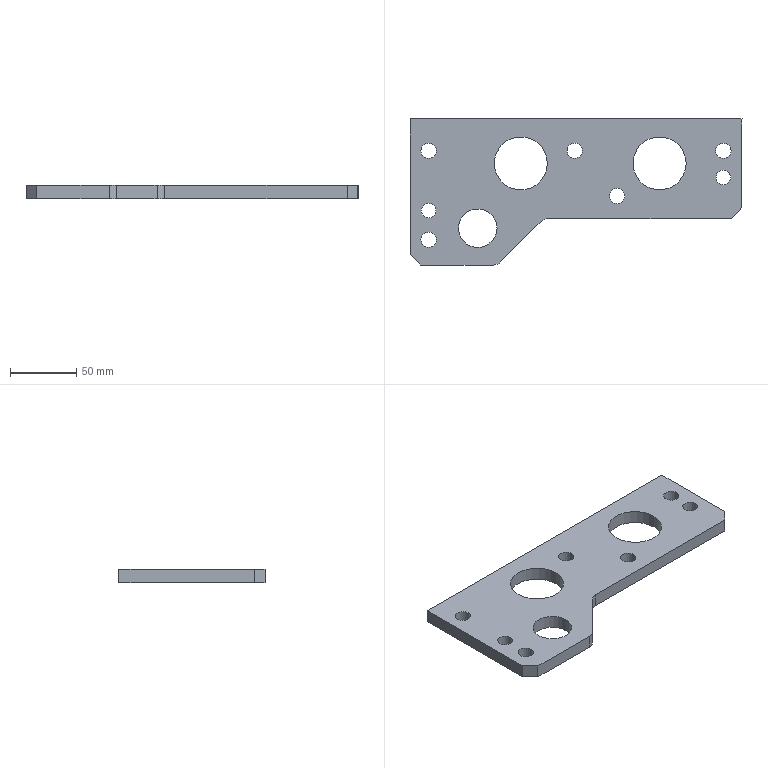Part | STEP file | lll_id4266_x_t | 1 solid | 22 faces | box 250 x 110 x 10 mm | volume 177245 mm3 | cylinder 12 | plane 10 | commonest cylinder face diameters 11.509 x5 11 x2 16 x2 40 x2 29 x1
STEP:
#1=CARTESIAN_POINT('',(3214.622,127.75,-35.));
#2=VERTEX_POINT('',#1);
#3=CARTESIAN_POINT('',(3214.622,127.75,-45.));
#4=VERTEX_POINT('',#3);
#5=CARTESIAN_POINT('',(3214.622,127.75,-35.));
#6=DIRECTION('',(0.,0.,-1.));
#7=VECTOR('',#6,1.);
#8=LINE('',#5,#7);
#9=EDGE_CURVE('',#2,#4,#8,.T.);
#10=ORIENTED_EDGE('',*,*,#9,.F.);
#11=CARTESIAN_POINT('',(3159.935,127.75,-35.));
#12=VERTEX_POINT('',#11);
#13=CARTESIAN_POINT('',(3266.435,127.75,-35.));
#14=DIRECTION('',(1.,0.,0.));
#15=VECTOR('',#14,1.);
#16=LINE('',#13,#15);
#17=EDGE_CURVE('',#12,#2,#16,.T.);
#18=ORIENTED_EDGE('',*,*,#17,.F.);
#19=CARTESIAN_POINT('',(3159.935,127.75,-45.));
#20=VERTEX_POINT('',#19);
#21=CARTESIAN_POINT('',(3159.935,127.75,-35.));
#22=DIRECTION('',(0.,0.,-1.));
#23=VECTOR('',#22,1.);
#24=LINE('',#21,#23);
#25=EDGE_CURVE('',#12,#20,#24,.T.);
#26=ORIENTED_EDGE('',*,*,#25,.T.);
#27=CARTESIAN_POINT('',(3266.435,127.75,-45.));
#28=DIRECTION('',(1.,0.,0.));
#29=VECTOR('',#28,1.);
#30=LINE('',#27,#29);
#31=EDGE_CURVE('',#20,#4,#30,.T.);
#32=ORIENTED_EDGE('',*,*,#31,.T.);
#33=EDGE_LOOP('',(#10,#18,#26,#32));
#34=FACE_OUTER_BOUND('',#33,.T.);
#35=CARTESIAN_POINT('',(3266.435,127.75,-35.));
#36=DIRECTION('',(0.,-1.,0.));
#37=DIRECTION('',(-1.,0.,0.));
#38=AXIS2_PLACEMENT_3D('',#35,#36,#37);
#39=PLANE('',#38);
#40=ADVANCED_FACE('',(#34),#39,.T.);
#41=ORIENTED_EDGE('',*,*,#25,.F.);
#42=CARTESIAN_POINT('',(3151.935,135.75,-35.));
#43=VERTEX_POINT('',#42);
#44=CARTESIAN_POINT('',(3169.435,118.25,-35.));
#45=DIRECTION('',(-0.7071,0.7071,0.));
#46=VECTOR('',#45,1.);
#47=LINE('',#44,#46);
#48=EDGE_CURVE('',#12,#43,#47,.T.);
#49=ORIENTED_EDGE('',*,*,#48,.T.);
#50=CARTESIAN_POINT('',(3151.935,135.75,-45.));
#51=VERTEX_POINT('',#50);
#52=CARTESIAN_POINT('',(3151.935,135.75,-35.));
#53=DIRECTION('',(0.,0.,-1.));
#54=VECTOR('',#53,1.);
#55=LINE('',#52,#54);
#56=EDGE_CURVE('',#43,#51,#55,.T.);
#57=ORIENTED_EDGE('',*,*,#56,.T.);
#58=CARTESIAN_POINT('',(3169.435,118.25,-45.));
#59=DIRECTION('',(-0.7071,0.7071,0.));
#60=VECTOR('',#59,1.);
#61=LINE('',#58,#60);
#62=EDGE_CURVE('',#20,#51,#61,.T.);
#63=ORIENTED_EDGE('',*,*,#62,.F.);
#64=EDGE_LOOP('',(#41,#49,#57,#63));
#65=FACE_OUTER_BOUND('',#64,.T.);
#66=CARTESIAN_POINT('',(3169.435,118.25,-35.));
#67=DIRECTION('',(-0.7071,-0.7071,0.));
#68=DIRECTION('',(-0.7071,0.7071,0.));
#69=AXIS2_PLACEMENT_3D('',#66,#67,#68);
#70=PLANE('',#69);
#71=ADVANCED_FACE('',(#65),#70,.T.);
#72=ORIENTED_EDGE('',*,*,#56,.F.);
#73=CARTESIAN_POINT('',(3151.935,237.75,-35.));
#74=VERTEX_POINT('',#73);
#75=CARTESIAN_POINT('',(3151.935,215.25,-35.));
#76=DIRECTION('',(0.,-1.,0.));
#77=VECTOR('',#76,1.);
#78=LINE('',#75,#77);
#79=EDGE_CURVE('',#74,#43,#78,.T.);
#80=ORIENTED_EDGE('',*,*,#79,.F.);
#81=CARTESIAN_POINT('',(3151.935,237.75,-45.));
#82=VERTEX_POINT('',#81);
#83=CARTESIAN_POINT('',(3151.935,237.75,-35.));
#84=DIRECTION('',(0.,0.,-1.));
#85=VECTOR('',#84,1.);
#86=LINE('',#83,#85);
#87=EDGE_CURVE('',#74,#82,#86,.T.);
#88=ORIENTED_EDGE('',*,*,#87,.T.);
#89=CARTESIAN_POINT('',(3151.935,215.25,-45.));
#90=DIRECTION('',(0.,-1.,0.));
#91=VECTOR('',#90,1.);
#92=LINE('',#89,#91);
#93=EDGE_CURVE('',#82,#51,#92,.T.);
#94=ORIENTED_EDGE('',*,*,#93,.T.);
#95=EDGE_LOOP('',(#72,#80,#88,#94));
#96=FACE_OUTER_BOUND('',#95,.T.);
#97=CARTESIAN_POINT('',(3151.935,215.25,-35.));
#98=DIRECTION('',(1.,0.,0.));
#99=DIRECTION('',(0.,-1.,0.));
#100=AXIS2_PLACEMENT_3D('',#97,#98,#99);
#101=PLANE('',#100);
#102=ADVANCED_FACE('',(#96),#101,.F.);
#103=ORIENTED_EDGE('',*,*,#87,.F.);
#104=CARTESIAN_POINT('',(3401.935,237.75,-35.));
#105=VERTEX_POINT('',#104);
#106=CARTESIAN_POINT('',(3266.435,237.75,-35.));
#107=DIRECTION('',(-1.,0.,0.));
#108=VECTOR('',#107,1.);
#109=LINE('',#106,#108);
#110=EDGE_CURVE('',#105,#74,#109,.T.);
#111=ORIENTED_EDGE('',*,*,#110,.F.);
#112=CARTESIAN_POINT('',(3401.935,237.75,-45.));
#113=VERTEX_POINT('',#112);
#114=CARTESIAN_POINT('',(3401.935,237.75,-35.));
#115=DIRECTION('',(0.,0.,-1.));
#116=VECTOR('',#115,1.);
#117=LINE('',#114,#116);
#118=EDGE_CURVE('',#105,#113,#117,.T.);
#119=ORIENTED_EDGE('',*,*,#118,.T.);
#120=CARTESIAN_POINT('',(3266.435,237.75,-45.));
#121=DIRECTION('',(-1.,0.,0.));
#122=VECTOR('',#121,1.);
#123=LINE('',#120,#122);
#124=EDGE_CURVE('',#113,#82,#123,.T.);
#125=ORIENTED_EDGE('',*,*,#124,.T.);
#126=EDGE_LOOP('',(#103,#111,#119,#125));
#127=FACE_OUTER_BOUND('',#126,.T.);
#128=CARTESIAN_POINT('',(3266.435,237.75,-35.));
#129=DIRECTION('',(0.,-1.,0.));
#130=DIRECTION('',(-1.,0.,0.));
#131=AXIS2_PLACEMENT_3D('',#128,#129,#130);
#132=PLANE('',#131);
#133=ADVANCED_FACE('',(#127),#132,.F.);
#134=ORIENTED_EDGE('',*,*,#118,.F.);
#135=CARTESIAN_POINT('',(3401.935,170.75,-35.));
#136=VERTEX_POINT('',#135);
#137=CARTESIAN_POINT('',(3401.935,215.25,-35.));
#138=DIRECTION('',(0.,1.,0.));
#139=VECTOR('',#138,1.);
#140=LINE('',#137,#139);
#141=EDGE_CURVE('',#136,#105,#140,.T.);
#142=ORIENTED_EDGE('',*,*,#141,.F.);
#143=CARTESIAN_POINT('',(3401.935,170.75,-45.));
#144=VERTEX_POINT('',#143);
#145=CARTESIAN_POINT('',(3401.935,170.75,-35.));
#146=DIRECTION('',(0.,0.,-1.));
#147=VECTOR('',#146,1.);
#148=LINE('',#145,#147);
#149=EDGE_CURVE('',#136,#144,#148,.T.);
#150=ORIENTED_EDGE('',*,*,#149,.T.);
#151=CARTESIAN_POINT('',(3401.935,215.25,-45.));
#152=DIRECTION('',(0.,1.,0.));
#153=VECTOR('',#152,1.);
#154=LINE('',#151,#153);
#155=EDGE_CURVE('',#144,#113,#154,.T.);
#156=ORIENTED_EDGE('',*,*,#155,.T.);
#157=EDGE_LOOP('',(#134,#142,#150,#156));
#158=FACE_OUTER_BOUND('',#157,.T.);
#159=CARTESIAN_POINT('',(3401.935,215.25,-35.));
#160=DIRECTION('',(-1.,0.,0.));
#161=DIRECTION('',(0.,1.,0.));
#162=AXIS2_PLACEMENT_3D('',#159,#160,#161);
#163=PLANE('',#162);
#164=ADVANCED_FACE('',(#158),#163,.F.);
#165=ORIENTED_EDGE('',*,*,#149,.F.);
#166=CARTESIAN_POINT('',(3393.935,162.75,-35.));
#167=VERTEX_POINT('',#166);
#168=CARTESIAN_POINT('',(3356.435,125.25,-35.));
#169=DIRECTION('',(-0.7071,-0.7071,0.));
#170=VECTOR('',#169,1.);
#171=LINE('',#168,#170);
#172=EDGE_CURVE('',#136,#167,#171,.T.);
#173=ORIENTED_EDGE('',*,*,#172,.T.);
#174=CARTESIAN_POINT('',(3393.935,162.75,-45.));
#175=VERTEX_POINT('',#174);
#176=CARTESIAN_POINT('',(3393.935,162.75,-35.));
#177=DIRECTION('',(0.,0.,-1.));
#178=VECTOR('',#177,1.);
#179=LINE('',#176,#178);
#180=EDGE_CURVE('',#167,#175,#179,.T.);
#181=ORIENTED_EDGE('',*,*,#180,.T.);
#182=CARTESIAN_POINT('',(3356.435,125.25,-45.));
#183=DIRECTION('',(-0.7071,-0.7071,0.));
#184=VECTOR('',#183,1.);
#185=LINE('',#182,#184);
#186=EDGE_CURVE('',#144,#175,#185,.T.);
#187=ORIENTED_EDGE('',*,*,#186,.F.);
#188=EDGE_LOOP('',(#165,#173,#181,#187));
#189=FACE_OUTER_BOUND('',#188,.T.);
#190=CARTESIAN_POINT('',(3356.435,125.25,-35.));
#191=DIRECTION('',(0.7071,-0.7071,0.));
#192=DIRECTION('',(-0.7071,-0.7071,0.));
#193=AXIS2_PLACEMENT_3D('',#190,#191,#192);
#194=PLANE('',#193);
#195=ADVANCED_FACE('',(#189),#194,.T.);
#196=ORIENTED_EDGE('',*,*,#180,.F.);
#197=CARTESIAN_POINT('',(3256.249,162.75,-35.));
#198=VERTEX_POINT('',#197);
#199=CARTESIAN_POINT('',(3266.435,162.75,-35.));
#200=DIRECTION('',(-1.,0.,0.));
#201=VECTOR('',#200,1.);
#202=LINE('',#199,#201);
#203=EDGE_CURVE('',#167,#198,#202,.T.);
#204=ORIENTED_EDGE('',*,*,#203,.T.);
#205=CARTESIAN_POINT('',(3256.249,162.75,-45.));
#206=VERTEX_POINT('',#205);
#207=CARTESIAN_POINT('',(3256.249,162.75,-35.));
#208=DIRECTION('',(0.,0.,-1.));
#209=VECTOR('',#208,1.);
#210=LINE('',#207,#209);
#211=EDGE_CURVE('',#198,#206,#210,.T.);
#212=ORIENTED_EDGE('',*,*,#211,.T.);
#213=CARTESIAN_POINT('',(3266.435,162.75,-45.));
#214=DIRECTION('',(-1.,0.,0.));
#215=VECTOR('',#214,1.);
#216=LINE('',#213,#215);
#217=EDGE_CURVE('',#175,#206,#216,.T.);
#218=ORIENTED_EDGE('',*,*,#217,.F.);
#219=EDGE_LOOP('',(#196,#204,#212,#218));
#220=FACE_OUTER_BOUND('',#219,.T.);
#221=CARTESIAN_POINT('',(3266.435,162.75,-35.));
#222=DIRECTION('',(0.,-1.,0.));
#223=DIRECTION('',(-1.,0.,0.));
#224=AXIS2_PLACEMENT_3D('',#221,#222,#223);
#225=PLANE('',#224);
#226=ADVANCED_FACE('',(#220),#225,.T.);
#227=ORIENTED_EDGE('',*,*,#211,.F.);
#228=CARTESIAN_POINT('',(3250.592,160.407,-35.));
#229=VERTEX_POINT('',#228);
#230=CARTESIAN_POINT('',(3256.249,154.75,-35.));
#231=DIRECTION('',(0.,0.,1.));
#232=DIRECTION('',(-1.,0.,0.));
#233=AXIS2_PLACEMENT_3D('',#230,#231,#232);
#234=CIRCLE('',#233,8.);
#235=EDGE_CURVE('',#198,#229,#234,.T.);
#236=ORIENTED_EDGE('',*,*,#235,.T.);
#237=CARTESIAN_POINT('',(3250.592,160.407,-45.));
#238=VERTEX_POINT('',#237);
#239=CARTESIAN_POINT('',(3250.592,160.407,-35.));
#240=DIRECTION('',(0.,0.,-1.));
#241=VECTOR('',#240,1.);
#242=LINE('',#239,#241);
#243=EDGE_CURVE('',#229,#238,#242,.T.);
#244=ORIENTED_EDGE('',*,*,#243,.T.);
#245=CARTESIAN_POINT('',(3256.249,154.75,-45.));
#246=DIRECTION('',(0.,0.,1.));
#247=DIRECTION('',(-1.,0.,0.));
#248=AXIS2_PLACEMENT_3D('',#245,#246,#247);
#249=CIRCLE('',#248,8.);
#250=EDGE_CURVE('',#206,#238,#249,.T.);
#251=ORIENTED_EDGE('',*,*,#250,.F.);
#252=EDGE_LOOP('',(#227,#236,#244,#251));
#253=FACE_OUTER_BOUND('',#252,.T.);
#254=CARTESIAN_POINT('',(3256.249,154.75,-35.));
#255=DIRECTION('',(0.,0.,-1.));
#256=DIRECTION('',(-1.,0.,0.));
#257=AXIS2_PLACEMENT_3D('',#254,#255,#256);
#258=CYLINDRICAL_SURFACE('',#257,8.);
#259=ADVANCED_FACE('',(#253),#258,.F.);
#260=ORIENTED_EDGE('',*,*,#243,.F.);
#261=CARTESIAN_POINT('',(3220.278,130.093,-35.));
#262=VERTEX_POINT('',#261);
#263=CARTESIAN_POINT('',(3285.935,195.75,-35.));
#264=DIRECTION('',(0.7071,0.7071,0.));
#265=VECTOR('',#264,1.);
#266=LINE('',#263,#265);
#267=EDGE_CURVE('',#262,#229,#266,.T.);
#268=ORIENTED_EDGE('',*,*,#267,.F.);
#269=CARTESIAN_POINT('',(3220.278,130.093,-45.));
#270=VERTEX_POINT('',#269);
#271=CARTESIAN_POINT('',(3220.278,130.093,-35.));
#272=DIRECTION('',(0.,0.,-1.));
#273=VECTOR('',#272,1.);
#274=LINE('',#271,#273);
#275=EDGE_CURVE('',#262,#270,#274,.T.);
#276=ORIENTED_EDGE('',*,*,#275,.T.);
#277=CARTESIAN_POINT('',(3285.935,195.75,-45.));
#278=DIRECTION('',(0.7071,0.7071,0.));
#279=VECTOR('',#278,1.);
#280=LINE('',#277,#279);
#281=EDGE_CURVE('',#270,#238,#280,.T.);
#282=ORIENTED_EDGE('',*,*,#281,.T.);
#283=EDGE_LOOP('',(#260,#268,#276,#282));
#284=FACE_OUTER_BOUND('',#283,.T.);
#285=CARTESIAN_POINT('',(3285.935,195.75,-35.));
#286=DIRECTION('',(0.7071,-0.7071,0.));
#287=DIRECTION('',(-0.7071,-0.7071,0.));
#288=AXIS2_PLACEMENT_3D('',#285,#286,#287);
#289=PLANE('',#288);
#290=ADVANCED_FACE('',(#284),#289,.T.);
#291=CARTESIAN_POINT('',(3188.5,155.5,-45.));
#292=VERTEX_POINT('',#291);
#293=CARTESIAN_POINT('',(3203.,155.5,-45.));
#294=DIRECTION('',(0.,0.,1.));
#295=DIRECTION('',(-1.,0.,0.));
#296=AXIS2_PLACEMENT_3D('',#293,#294,#295);
#297=CIRCLE('',#296,14.5);
#298=EDGE_CURVE('',#292,#292,#297,.T.);
#299=ORIENTED_EDGE('',*,*,#298,.F.);
#300=EDGE_LOOP('',(#299));
#301=FACE_BOUND('',#300,.T.);
#302=CARTESIAN_POINT('',(3188.5,155.5,-35.));
#303=VERTEX_POINT('',#302);
#304=CARTESIAN_POINT('',(3203.,155.5,-35.));
#305=DIRECTION('',(0.,0.,1.));
#306=DIRECTION('',(-1.,0.,0.));
#307=AXIS2_PLACEMENT_3D('',#304,#305,#306);
#308=CIRCLE('',#307,14.5);
#309=EDGE_CURVE('',#303,#303,#308,.T.);
#310=ORIENTED_EDGE('',*,*,#309,.T.);
#311=EDGE_LOOP('',(#310));
#312=FACE_BOUND('',#311,.T.);
#313=CARTESIAN_POINT('',(3203.,155.5,-35.));
#314=DIRECTION('',(0.,0.,-1.));
#315=DIRECTION('',(-1.,0.,0.));
#316=AXIS2_PLACEMENT_3D('',#313,#314,#315);
#317=CYLINDRICAL_SURFACE('',#316,14.5);
#318=ADVANCED_FACE('',(#301,#312),#317,.F.);
#319=CARTESIAN_POINT('',(3393.69,213.75,-45.));
#320=VERTEX_POINT('',#319);
#321=CARTESIAN_POINT('',(3387.935,213.75,-45.));
#322=DIRECTION('',(0.,0.,1.));
#323=DIRECTION('',(1.,0.,0.));
#324=AXIS2_PLACEMENT_3D('',#321,#322,#323);
#325=CIRCLE('',#324,5.755);
#326=EDGE_CURVE('',#320,#320,#325,.T.);
#327=ORIENTED_EDGE('',*,*,#326,.F.);
#328=EDGE_LOOP('',(#327));
#329=FACE_BOUND('',#328,.T.);
#330=CARTESIAN_POINT('',(3382.181,213.75,-35.));
#331=VERTEX_POINT('',#330);
#332=CARTESIAN_POINT('',(3387.935,213.75,-35.));
#333=DIRECTION('',(0.,0.,1.));
#334=DIRECTION('',(-1.,0.,0.));
#335=AXIS2_PLACEMENT_3D('',#332,#333,#334);
#336=CIRCLE('',#335,5.755);
#337=EDGE_CURVE('',#331,#331,#336,.T.);
#338=ORIENTED_EDGE('',*,*,#337,.T.);
#339=EDGE_LOOP('',(#338));
#340=FACE_BOUND('',#339,.T.);
#341=CARTESIAN_POINT('',(3387.935,213.75,-35.));
#342=DIRECTION('',(0.,0.,1.));
#343=DIRECTION('',(1.,0.,0.));
#344=AXIS2_PLACEMENT_3D('',#341,#342,#343);
#345=CYLINDRICAL_SURFACE('',#344,5.755);
#346=ADVANCED_FACE('',(#329,#340),#345,.F.);
#347=CARTESIAN_POINT('',(3382.435,193.75,-45.));
#348=VERTEX_POINT('',#347);
#349=CARTESIAN_POINT('',(3387.935,193.75,-45.));
#350=DIRECTION('',(0.,0.,1.));
#351=DIRECTION('',(-1.,0.,0.));
#352=AXIS2_PLACEMENT_3D('',#349,#350,#351);
#353=CIRCLE('',#352,5.5);
#354=EDGE_CURVE('',#348,#348,#353,.T.);
#355=ORIENTED_EDGE('',*,*,#354,.F.);
#356=EDGE_LOOP('',(#355));
#357=FACE_BOUND('',#356,.T.);
#358=CARTESIAN_POINT('',(3382.435,193.75,-35.));
#359=VERTEX_POINT('',#358);
#360=CARTESIAN_POINT('',(3387.935,193.75,-35.));
#361=DIRECTION('',(0.,0.,1.));
#362=DIRECTION('',(-1.,0.,0.));
#363=AXIS2_PLACEMENT_3D('',#360,#361,#362);
#364=CIRCLE('',#363,5.5);
#365=EDGE_CURVE('',#359,#359,#364,.T.);
#366=ORIENTED_EDGE('',*,*,#365,.T.);
#367=EDGE_LOOP('',(#366));
#368=FACE_BOUND('',#367,.T.);
#369=CARTESIAN_POINT('',(3387.935,193.75,-35.));
#370=DIRECTION('',(0.,0.,1.));
#371=DIRECTION('',(1.,0.,0.));
#372=AXIS2_PLACEMENT_3D('',#369,#370,#371);
#373=CYLINDRICAL_SURFACE('',#372,5.5);
#374=ADVANCED_FACE('',(#357,#368),#373,.F.);
#375=CARTESIAN_POINT('',(3313.69,179.75,-45.));
#376=VERTEX_POINT('',#375);
#377=CARTESIAN_POINT('',(3307.935,179.75,-45.));
#378=DIRECTION('',(0.,0.,1.));
#379=DIRECTION('',(1.,0.,0.));
#380=AXIS2_PLACEMENT_3D('',#377,#378,#379);
#381=CIRCLE('',#380,5.755);
#382=EDGE_CURVE('',#376,#376,#381,.T.);
#383=ORIENTED_EDGE('',*,*,#382,.F.);
#384=EDGE_LOOP('',(#383));
#385=FACE_BOUND('',#384,.T.);
#386=CARTESIAN_POINT('',(3302.181,179.75,-35.));
#387=VERTEX_POINT('',#386);
#388=CARTESIAN_POINT('',(3307.935,179.75,-35.));
#389=DIRECTION('',(0.,0.,1.));
#390=DIRECTION('',(-1.,0.,0.));
#391=AXIS2_PLACEMENT_3D('',#388,#389,#390);
#392=CIRCLE('',#391,5.755);
#393=EDGE_CURVE('',#387,#387,#392,.T.);
#394=ORIENTED_EDGE('',*,*,#393,.T.);
#395=EDGE_LOOP('',(#394));
#396=FACE_BOUND('',#395,.T.);
#397=CARTESIAN_POINT('',(3307.935,179.75,-35.));
#398=DIRECTION('',(0.,0.,1.));
#399=DIRECTION('',(1.,0.,0.));
#400=AXIS2_PLACEMENT_3D('',#397,#398,#399);
#401=CYLINDRICAL_SURFACE('',#400,5.755);
#402=ADVANCED_FACE('',(#385,#396),#401,.F.);
#403=CARTESIAN_POINT('',(3281.69,213.75,-45.));
#404=VERTEX_POINT('',#403);
#405=CARTESIAN_POINT('',(3275.935,213.75,-45.));
#406=DIRECTION('',(0.,0.,1.));
#407=DIRECTION('',(1.,0.,0.));
#408=AXIS2_PLACEMENT_3D('',#405,#406,#407);
#409=CIRCLE('',#408,5.755);
#410=EDGE_CURVE('',#404,#404,#409,.T.);
#411=ORIENTED_EDGE('',*,*,#410,.F.);
#412=EDGE_LOOP('',(#411));
#413=FACE_BOUND('',#412,.T.);
#414=CARTESIAN_POINT('',(3270.181,213.75,-35.));
#415=VERTEX_POINT('',#414);
#416=CARTESIAN_POINT('',(3275.935,213.75,-35.));
#417=DIRECTION('',(0.,0.,1.));
#418=DIRECTION('',(-1.,0.,0.));
#419=AXIS2_PLACEMENT_3D('',#416,#417,#418);
#420=CIRCLE('',#419,5.755);
#421=EDGE_CURVE('',#415,#415,#420,.T.);
#422=ORIENTED_EDGE('',*,*,#421,.T.);
#423=EDGE_LOOP('',(#422));
#424=FACE_BOUND('',#423,.T.);
#425=CARTESIAN_POINT('',(3275.935,213.75,-35.));
#426=DIRECTION('',(0.,0.,1.));
#427=DIRECTION('',(1.,0.,0.));
#428=AXIS2_PLACEMENT_3D('',#425,#426,#427);
#429=CYLINDRICAL_SURFACE('',#428,5.755);
#430=ADVANCED_FACE('',(#413,#424),#429,.F.);
#431=CARTESIAN_POINT('',(3160.435,168.75,-45.));
#432=VERTEX_POINT('',#431);
#433=CARTESIAN_POINT('',(3165.935,168.75,-45.));
#434=DIRECTION('',(0.,0.,1.));
#435=DIRECTION('',(-1.,0.,0.));
#436=AXIS2_PLACEMENT_3D('',#433,#434,#435);
#437=CIRCLE('',#436,5.5);
#438=EDGE_CURVE('',#432,#432,#437,.T.);
#439=ORIENTED_EDGE('',*,*,#438,.F.);
#440=EDGE_LOOP('',(#439));
#441=FACE_BOUND('',#440,.T.);
#442=CARTESIAN_POINT('',(3160.435,168.75,-35.));
#443=VERTEX_POINT('',#442);
#444=CARTESIAN_POINT('',(3165.935,168.75,-35.));
#445=DIRECTION('',(0.,0.,1.));
#446=DIRECTION('',(-1.,0.,0.));
#447=AXIS2_PLACEMENT_3D('',#444,#445,#446);
#448=CIRCLE('',#447,5.5);
#449=EDGE_CURVE('',#443,#443,#448,.T.);
#450=ORIENTED_EDGE('',*,*,#449,.T.);
#451=EDGE_LOOP('',(#450));
#452=FACE_BOUND('',#451,.T.);
#453=CARTESIAN_POINT('',(3165.935,168.75,-35.));
#454=DIRECTION('',(0.,0.,1.));
#455=DIRECTION('',(1.,0.,0.));
#456=AXIS2_PLACEMENT_3D('',#453,#454,#455);
#457=CYLINDRICAL_SURFACE('',#456,5.5);
#458=ADVANCED_FACE('',(#441,#452),#457,.F.);
#459=CARTESIAN_POINT('',(3171.69,213.75,-45.));
#460=VERTEX_POINT('',#459);
#461=CARTESIAN_POINT('',(3165.935,213.75,-45.));
#462=DIRECTION('',(0.,0.,1.));
#463=DIRECTION('',(1.,0.,0.));
#464=AXIS2_PLACEMENT_3D('',#461,#462,#463);
#465=CIRCLE('',#464,5.755);
#466=EDGE_CURVE('',#460,#460,#465,.T.);
#467=ORIENTED_EDGE('',*,*,#466,.F.);
#468=EDGE_LOOP('',(#467));
#469=FACE_BOUND('',#468,.T.);
#470=CARTESIAN_POINT('',(3160.181,213.75,-35.));
#471=VERTEX_POINT('',#470);
#472=CARTESIAN_POINT('',(3165.935,213.75,-35.));
#473=DIRECTION('',(0.,0.,1.));
#474=DIRECTION('',(-1.,0.,0.));
#475=AXIS2_PLACEMENT_3D('',#472,#473,#474);
#476=CIRCLE('',#475,5.755);
#477=EDGE_CURVE('',#471,#471,#476,.T.);
#478=ORIENTED_EDGE('',*,*,#477,.T.);
#479=EDGE_LOOP('',(#478));
#480=FACE_BOUND('',#479,.T.);
#481=CARTESIAN_POINT('',(3165.935,213.75,-35.));
#482=DIRECTION('',(0.,0.,1.));
#483=DIRECTION('',(1.,0.,0.));
#484=AXIS2_PLACEMENT_3D('',#481,#482,#483);
#485=CYLINDRICAL_SURFACE('',#484,5.755);
#486=ADVANCED_FACE('',(#469,#480),#485,.F.);
#487=CARTESIAN_POINT('',(3171.69,146.75,-45.));
#488=VERTEX_POINT('',#487);
#489=CARTESIAN_POINT('',(3165.935,146.75,-45.));
#490=DIRECTION('',(0.,0.,1.));
#491=DIRECTION('',(1.,0.,0.));
#492=AXIS2_PLACEMENT_3D('',#489,#490,#491);
#493=CIRCLE('',#492,5.755);
#494=EDGE_CURVE('',#488,#488,#493,.T.);
#495=ORIENTED_EDGE('',*,*,#494,.F.);
#496=EDGE_LOOP('',(#495));
#497=FACE_BOUND('',#496,.T.);
#498=CARTESIAN_POINT('',(3160.181,146.75,-35.));
#499=VERTEX_POINT('',#498);
#500=CARTESIAN_POINT('',(3165.935,146.75,-35.));
#501=DIRECTION('',(0.,0.,1.));
#502=DIRECTION('',(-1.,0.,0.));
#503=AXIS2_PLACEMENT_3D('',#500,#501,#502);
#504=CIRCLE('',#503,5.755);
#505=EDGE_CURVE('',#499,#499,#504,.T.);
#506=ORIENTED_EDGE('',*,*,#505,.T.);
#507=EDGE_LOOP('',(#506));
#508=FACE_BOUND('',#507,.T.);
#509=CARTESIAN_POINT('',(3165.935,146.75,-35.));
#510=DIRECTION('',(0.,0.,1.));
#511=DIRECTION('',(1.,0.,0.));
#512=AXIS2_PLACEMENT_3D('',#509,#510,#511);
#513=CYLINDRICAL_SURFACE('',#512,5.755);
#514=ADVANCED_FACE('',(#497,#508),#513,.F.);
#515=CARTESIAN_POINT('',(3214.622,135.75,-35.));
#516=DIRECTION('',(0.,0.,-1.));
#517=DIRECTION('',(-1.,0.,0.));
#518=AXIS2_PLACEMENT_3D('',#515,#516,#517);
#519=CIRCLE('',#518,8.);
#520=EDGE_CURVE('',#262,#2,#519,.T.);
#521=ORIENTED_EDGE('',*,*,#520,.T.);
#522=ORIENTED_EDGE('',*,*,#9,.T.);
#523=CARTESIAN_POINT('',(3214.622,135.75,-45.));
#524=DIRECTION('',(0.,0.,-1.));
#525=DIRECTION('',(-1.,0.,0.));
#526=AXIS2_PLACEMENT_3D('',#523,#524,#525);
#527=CIRCLE('',#526,8.);
#528=EDGE_CURVE('',#270,#4,#527,.T.);
#529=ORIENTED_EDGE('',*,*,#528,.F.);
#530=ORIENTED_EDGE('',*,*,#275,.F.);
#531=EDGE_LOOP('',(#521,#522,#529,#530));
#532=FACE_OUTER_BOUND('',#531,.T.);
#533=CARTESIAN_POINT('',(3214.622,135.75,-35.));
#534=DIRECTION('',(0.,0.,-1.));
#535=DIRECTION('',(-1.,0.,0.));
#536=AXIS2_PLACEMENT_3D('',#533,#534,#535);
#537=CYLINDRICAL_SURFACE('',#536,8.);
#538=ADVANCED_FACE('',(#532),#537,.T.);
#539=CARTESIAN_POINT('',(3215.367,204.288,-45.));
#540=VERTEX_POINT('',#539);
#541=CARTESIAN_POINT('',(3235.367,204.288,-45.));
#542=DIRECTION('',(0.,0.,-1.));
#543=DIRECTION('',(-1.,0.,0.));
#544=AXIS2_PLACEMENT_3D('',#541,#542,#543);
#545=CIRCLE('',#544,20.);
#546=EDGE_CURVE('',#540,#540,#545,.T.);
#547=ORIENTED_EDGE('',*,*,#546,.T.);
#548=EDGE_LOOP('',(#547));
#549=FACE_BOUND('',#548,.T.);
#550=CARTESIAN_POINT('',(3215.367,204.288,-35.));
#551=VERTEX_POINT('',#550);
#552=CARTESIAN_POINT('',(3235.367,204.288,-35.));
#553=DIRECTION('',(0.,0.,-1.));
#554=DIRECTION('',(-1.,0.,0.));
#555=AXIS2_PLACEMENT_3D('',#552,#553,#554);
#556=CIRCLE('',#555,20.);
#557=EDGE_CURVE('',#551,#551,#556,.T.);
#558=ORIENTED_EDGE('',*,*,#557,.F.);
#559=EDGE_LOOP('',(#558));
#560=FACE_BOUND('',#559,.T.);
#561=CARTESIAN_POINT('',(3235.367,204.288,-35.));
#562=DIRECTION('',(0.,0.,1.));
#563=DIRECTION('',(1.,0.,0.));
#564=AXIS2_PLACEMENT_3D('',#561,#562,#563);
#565=CYLINDRICAL_SURFACE('',#564,20.);
#566=ADVANCED_FACE('',(#549,#560),#565,.F.);
#567=CARTESIAN_POINT('',(3319.867,204.288,-45.));
#568=VERTEX_POINT('',#567);
#569=CARTESIAN_POINT('',(3339.867,204.288,-45.));
#570=DIRECTION('',(0.,0.,-1.));
#571=DIRECTION('',(-1.,0.,0.));
#572=AXIS2_PLACEMENT_3D('',#569,#570,#571);
#573=CIRCLE('',#572,20.);
#574=EDGE_CURVE('',#568,#568,#573,.T.);
#575=ORIENTED_EDGE('',*,*,#574,.T.);
#576=EDGE_LOOP('',(#575));
#577=FACE_BOUND('',#576,.T.);
#578=CARTESIAN_POINT('',(3319.867,204.288,-35.));
#579=VERTEX_POINT('',#578);
#580=CARTESIAN_POINT('',(3339.867,204.288,-35.));
#581=DIRECTION('',(0.,0.,-1.));
#582=DIRECTION('',(-1.,0.,0.));
#583=AXIS2_PLACEMENT_3D('',#580,#581,#582);
#584=CIRCLE('',#583,20.);
#585=EDGE_CURVE('',#579,#579,#584,.T.);
#586=ORIENTED_EDGE('',*,*,#585,.F.);
#587=EDGE_LOOP('',(#586));
#588=FACE_BOUND('',#587,.T.);
#589=CARTESIAN_POINT('',(3339.867,204.288,-35.));
#590=DIRECTION('',(0.,0.,1.));
#591=DIRECTION('',(1.,0.,0.));
#592=AXIS2_PLACEMENT_3D('',#589,#590,#591);
#593=CYLINDRICAL_SURFACE('',#592,20.);
#594=ADVANCED_FACE('',(#577,#588),#593,.F.);
#595=ORIENTED_EDGE('',*,*,#298,.T.);
#596=EDGE_LOOP('',(#595));
#597=FACE_BOUND('',#596,.T.);
#598=ORIENTED_EDGE('',*,*,#326,.T.);
#599=EDGE_LOOP('',(#598));
#600=FACE_BOUND('',#599,.T.);
#601=ORIENTED_EDGE('',*,*,#354,.T.);
#602=EDGE_LOOP('',(#601));
#603=FACE_BOUND('',#602,.T.);
#604=ORIENTED_EDGE('',*,*,#382,.T.);
#605=EDGE_LOOP('',(#604));
#606=FACE_BOUND('',#605,.T.);
#607=ORIENTED_EDGE('',*,*,#410,.T.);
#608=EDGE_LOOP('',(#607));
#609=FACE_BOUND('',#608,.T.);
#610=ORIENTED_EDGE('',*,*,#438,.T.);
#611=EDGE_LOOP('',(#610));
#612=FACE_BOUND('',#611,.T.);
#613=ORIENTED_EDGE('',*,*,#466,.T.);
#614=EDGE_LOOP('',(#613));
#615=FACE_BOUND('',#614,.T.);
#616=ORIENTED_EDGE('',*,*,#494,.T.);
#617=EDGE_LOOP('',(#616));
#618=FACE_BOUND('',#617,.T.);
#619=ORIENTED_EDGE('',*,*,#281,.F.);
#620=ORIENTED_EDGE('',*,*,#528,.T.);
#621=ORIENTED_EDGE('',*,*,#31,.F.);
#622=ORIENTED_EDGE('',*,*,#62,.T.);
#623=ORIENTED_EDGE('',*,*,#93,.F.);
#624=ORIENTED_EDGE('',*,*,#124,.F.);
#625=ORIENTED_EDGE('',*,*,#155,.F.);
#626=ORIENTED_EDGE('',*,*,#186,.T.);
#627=ORIENTED_EDGE('',*,*,#217,.T.);
#628=ORIENTED_EDGE('',*,*,#250,.T.);
#629=EDGE_LOOP('',(#619,#620,#621,#622,#623,#624,#625,#626,#627,#628));
#630=FACE_BOUND('',#629,.T.);
#631=ORIENTED_EDGE('',*,*,#546,.F.);
#632=EDGE_LOOP('',(#631));
#633=FACE_BOUND('',#632,.T.);
#634=ORIENTED_EDGE('',*,*,#574,.F.);
#635=EDGE_LOOP('',(#634));
#636=FACE_BOUND('',#635,.T.);
#637=CARTESIAN_POINT('',(3266.435,215.25,-45.));
#638=DIRECTION('',(0.,0.,-1.));
#639=DIRECTION('',(1.,0.,0.));
#640=AXIS2_PLACEMENT_3D('',#637,#638,#639);
#641=PLANE('',#640);
#642=ADVANCED_FACE('',(#597,#600,#603,#606,#609,#612,#615,#618,#630,#633,#636),#641,.T.);
#643=ORIENTED_EDGE('',*,*,#309,.F.);
#644=EDGE_LOOP('',(#643));
#645=FACE_BOUND('',#644,.T.);
#646=ORIENTED_EDGE('',*,*,#337,.F.);
#647=EDGE_LOOP('',(#646));
#648=FACE_BOUND('',#647,.T.);
#649=ORIENTED_EDGE('',*,*,#365,.F.);
#650=EDGE_LOOP('',(#649));
#651=FACE_BOUND('',#650,.T.);
#652=ORIENTED_EDGE('',*,*,#393,.F.);
#653=EDGE_LOOP('',(#652));
#654=FACE_BOUND('',#653,.T.);
#655=ORIENTED_EDGE('',*,*,#421,.F.);
#656=EDGE_LOOP('',(#655));
#657=FACE_BOUND('',#656,.T.);
#658=ORIENTED_EDGE('',*,*,#449,.F.);
#659=EDGE_LOOP('',(#658));
#660=FACE_BOUND('',#659,.T.);
#661=ORIENTED_EDGE('',*,*,#477,.F.);
#662=EDGE_LOOP('',(#661));
#663=FACE_BOUND('',#662,.T.);
#664=ORIENTED_EDGE('',*,*,#505,.F.);
#665=EDGE_LOOP('',(#664));
#666=FACE_BOUND('',#665,.T.);
#667=ORIENTED_EDGE('',*,*,#267,.T.);
#668=ORIENTED_EDGE('',*,*,#235,.F.);
#669=ORIENTED_EDGE('',*,*,#203,.F.);
#670=ORIENTED_EDGE('',*,*,#172,.F.);
#671=ORIENTED_EDGE('',*,*,#141,.T.);
#672=ORIENTED_EDGE('',*,*,#110,.T.);
#673=ORIENTED_EDGE('',*,*,#79,.T.);
#674=ORIENTED_EDGE('',*,*,#48,.F.);
#675=ORIENTED_EDGE('',*,*,#17,.T.);
#676=ORIENTED_EDGE('',*,*,#520,.F.);
#677=EDGE_LOOP('',(#667,#668,#669,#670,#671,#672,#673,#674,#675,#676));
#678=FACE_BOUND('',#677,.T.);
#679=ORIENTED_EDGE('',*,*,#557,.T.);
#680=EDGE_LOOP('',(#679));
#681=FACE_BOUND('',#680,.T.);
#682=ORIENTED_EDGE('',*,*,#585,.T.);
#683=EDGE_LOOP('',(#682));
#684=FACE_BOUND('',#683,.T.);
#685=CARTESIAN_POINT('',(3266.435,215.25,-35.));
#686=DIRECTION('',(0.,0.,-1.));
#687=DIRECTION('',(1.,0.,0.));
#688=AXIS2_PLACEMENT_3D('',#685,#686,#687);
#689=PLANE('',#688);
#690=ADVANCED_FACE('',(#645,#648,#651,#654,#657,#660,#663,#666,#678,#681,#684),#689,.F.);
#691=CLOSED_SHELL('',(#40,#71,#102,#133,#164,#195,#226,#259,#290,#318,#346,#374,#402,#430,#458,#486,#514,#538,#566,#594,#642,#690));
#692=MANIFOLD_SOLID_BREP('',#691);
#693=(LENGTH_UNIT()NAMED_UNIT(*)SI_UNIT(.MILLI.,.METRE.));
#694=UNCERTAINTY_MEASURE_WITH_UNIT(LENGTH_MEASURE(0.00002),#693,'','');
#695=(NAMED_UNIT(*)PLANE_ANGLE_UNIT()SI_UNIT($,.RADIAN.));
#696=PLANE_ANGLE_MEASURE_WITH_UNIT(PLANE_ANGLE_MEASURE(0.01745),#695);
#697=DIMENSIONAL_EXPONENTS(0.,0.,0.,0.,0.,0.,0.);
#698=(CONVERSION_BASED_UNIT('DEGREE',#696)NAMED_UNIT(#697)PLANE_ANGLE_UNIT());
#699=(NAMED_UNIT(*)SI_UNIT($,.STERADIAN.)SOLID_ANGLE_UNIT());
#700=(GEOMETRIC_REPRESENTATION_CONTEXT(3)GLOBAL_UNCERTAINTY_ASSIGNED_CONTEXT((#694))GLOBAL_UNIT_ASSIGNED_CONTEXT((#693,#698,#699))REPRESENTATION_CONTEXT('',''));
#701=ADVANCED_BREP_SHAPE_REPRESENTATION('',(#692),#700);